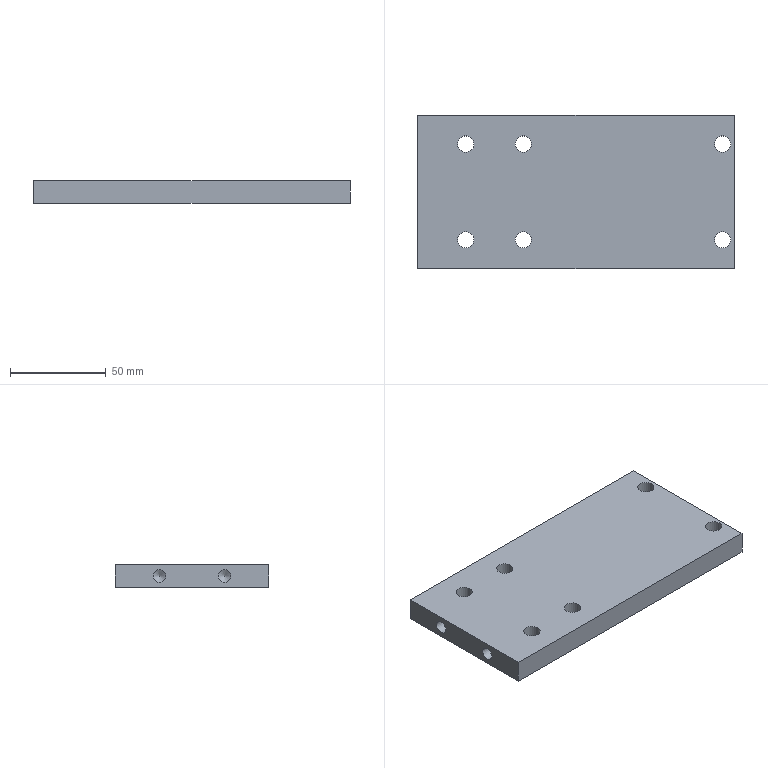Part | STEP file | SUPORTE | 1 solid | 16 faces | box 165 x 80 x 12 mm | volume 153227 mm3 | cylinder 8 | plane 6 | cone 2 | commonest cylinder face diameters 8.5 x6 6.647 x2
STEP:
#1=CARTESIAN_POINT('',(0.,0.,0.));
#2=DIRECTION('',(0.,0.,1.));
#3=DIRECTION('',(1.,0.,0.));
#4=AXIS2_PLACEMENT_3D('',#1,#2,#3);
#5=CARTESIAN_POINT('',(-206.95,452.,9.323));
#6=VERTEX_POINT('',#5);
#7=CARTESIAN_POINT('',(-206.95,452.,6.));
#8=DIRECTION('',(-1.,0.,0.));
#9=DIRECTION('',(0.,0.,1.));
#10=AXIS2_PLACEMENT_3D('',#7,#8,#9);
#11=CIRCLE('',#10,3.324);
#12=CARTESIAN_POINT('',(-205.952,452.,6.));
#13=DIRECTION('',(-1.,0.,0.));
#14=DIRECTION('',(0.,0.,1.));
#15=AXIS2_PLACEMENT_3D('',#12,#13,#14);
#16=CONICAL_SURFACE('',#15,1.662,1.03);
#17=CARTESIAN_POINT('',(0.,0.9985));
#18=DIRECTION('',(1.,0.));
#19=VECTOR('',#18,1.);
#20=LINE('',#17,#19);
#21=(GEOMETRIC_REPRESENTATION_CONTEXT(2)PARAMETRIC_REPRESENTATION_CONTEXT()REPRESENTATION_CONTEXT('',''));
#22=DEFINITIONAL_REPRESENTATION('',(#20),#21);
#23=PCURVE('',#16,#22);
#24=CARTESIAN_POINT('',(-214.45,452.,6.));
#25=DIRECTION('',(-1.,0.,0.));
#26=DIRECTION('',(0.,0.,1.));
#27=AXIS2_PLACEMENT_3D('',#24,#25,#26);
#28=CYLINDRICAL_SURFACE('',#27,3.324);
#29=CARTESIAN_POINT('',(0.,-7.5));
#30=DIRECTION('',(1.,0.));
#31=VECTOR('',#30,1.);
#32=LINE('',#29,#31);
#33=(GEOMETRIC_REPRESENTATION_CONTEXT(2)PARAMETRIC_REPRESENTATION_CONTEXT()REPRESENTATION_CONTEXT('',''));
#34=DEFINITIONAL_REPRESENTATION('',(#32),#33);
#35=PCURVE('',#28,#34);
#36=SURFACE_CURVE('',#11,(#23,#35),.PCURVE_S1.);
#37=EDGE_CURVE('',#6,#6,#36,.T.);
#38=ORIENTED_EDGE('',*,*,#37,.F.);
#39=CARTESIAN_POINT('',(-204.953,452.,6.));
#40=VERTEX_POINT('',#39);
#41=CARTESIAN_POINT('',(-204.953,452.,6.));
#42=CARTESIAN_POINT('',(-206.95,452.,9.323));
#43=B_SPLINE_CURVE_WITH_KNOTS('',1,(#41,#42),.UNSPECIFIED.,.F.,.F.,(2,2),(-1.939,1.939),.PIECEWISE_BEZIER_KNOTS.);
#44=CARTESIAN_POINT('',(0.,0.));
#45=DIRECTION('',(0.,1.));
#46=VECTOR('',#45,1.);
#47=LINE('',#44,#46);
#48=(GEOMETRIC_REPRESENTATION_CONTEXT(2)PARAMETRIC_REPRESENTATION_CONTEXT()REPRESENTATION_CONTEXT('',''));
#49=DEFINITIONAL_REPRESENTATION('',(#47),#48);
#50=PCURVE('',#16,#49);
#51=CARTESIAN_POINT('',(6.283,0.));
#52=DIRECTION('',(0.,1.));
#53=VECTOR('',#52,1.);
#54=LINE('',#51,#53);
#55=(GEOMETRIC_REPRESENTATION_CONTEXT(2)PARAMETRIC_REPRESENTATION_CONTEXT()REPRESENTATION_CONTEXT('',''));
#56=DEFINITIONAL_REPRESENTATION('',(#54),#55);
#57=PCURVE('',#16,#56);
#58=SEAM_CURVE('',#43,(#50,#57),.PCURVE_S1.);
#59=EDGE_CURVE('',#40,#6,#58,.T.);
#60=ORIENTED_EDGE('',*,*,#59,.F.);
#61=ORIENTED_EDGE('',*,*,#59,.T.);
#62=EDGE_LOOP('',(#38,#60,#61));
#63=FACE_BOUND('',#62,.F.);
#64=ADVANCED_FACE('',(#63),#16,.F.);
#65=CARTESIAN_POINT('',(-221.95,452.,9.323));
#66=VERTEX_POINT('',#65);
#67=CARTESIAN_POINT('',(-221.95,452.,6.));
#68=DIRECTION('',(1.,0.,0.));
#69=DIRECTION('',(0.,0.,1.));
#70=AXIS2_PLACEMENT_3D('',#67,#68,#69);
#71=CIRCLE('',#70,3.324);
#72=CARTESIAN_POINT('',(6.283,7.5));
#73=DIRECTION('',(-1.,0.));
#74=VECTOR('',#73,1.);
#75=LINE('',#72,#74);
#76=(GEOMETRIC_REPRESENTATION_CONTEXT(2)PARAMETRIC_REPRESENTATION_CONTEXT()REPRESENTATION_CONTEXT('',''));
#77=DEFINITIONAL_REPRESENTATION('',(#75),#76);
#78=PCURVE('',#28,#77);
#79=CARTESIAN_POINT('',(-221.95,435.,6.));
#80=DIRECTION('',(1.,0.,0.));
#81=DIRECTION('',(0.,0.,-1.));
#82=AXIS2_PLACEMENT_3D('',#79,#80,#81);
#83=PLANE('',#82);
#84=CARTESIAN_POINT('',(0.,17.));
#85=DIRECTION('',(-1.,0.));
#86=AXIS2_PLACEMENT_2D('',#84,#85);
#87=CIRCLE('',#86,3.324);
#88=(GEOMETRIC_REPRESENTATION_CONTEXT(2)PARAMETRIC_REPRESENTATION_CONTEXT()REPRESENTATION_CONTEXT('',''));
#89=DEFINITIONAL_REPRESENTATION('',(#87),#88);
#90=PCURVE('',#83,#89);
#91=SURFACE_CURVE('',#71,(#78,#90),.PCURVE_S1.);
#92=EDGE_CURVE('',#66,#66,#91,.T.);
#93=ORIENTED_EDGE('',*,*,#92,.T.);
#94=CARTESIAN_POINT('',(-206.95,452.,9.323));
#95=CARTESIAN_POINT('',(-221.95,452.,9.323));
#96=B_SPLINE_CURVE_WITH_KNOTS('',1,(#94,#95),.UNSPECIFIED.,.F.,.F.,(2,2),(-7.5,7.5),.PIECEWISE_BEZIER_KNOTS.);
#97=CARTESIAN_POINT('',(0.,0.));
#98=DIRECTION('',(0.,1.));
#99=VECTOR('',#98,1.);
#100=LINE('',#97,#99);
#101=(GEOMETRIC_REPRESENTATION_CONTEXT(2)PARAMETRIC_REPRESENTATION_CONTEXT()REPRESENTATION_CONTEXT('',''));
#102=DEFINITIONAL_REPRESENTATION('',(#100),#101);
#103=PCURVE('',#28,#102);
#104=CARTESIAN_POINT('',(6.283,0.));
#105=DIRECTION('',(0.,1.));
#106=VECTOR('',#105,1.);
#107=LINE('',#104,#106);
#108=(GEOMETRIC_REPRESENTATION_CONTEXT(2)PARAMETRIC_REPRESENTATION_CONTEXT()REPRESENTATION_CONTEXT('',''));
#109=DEFINITIONAL_REPRESENTATION('',(#107),#108);
#110=PCURVE('',#28,#109);
#111=SEAM_CURVE('',#96,(#103,#110),.PCURVE_S1.);
#112=EDGE_CURVE('',#6,#66,#111,.T.);
#113=ORIENTED_EDGE('',*,*,#112,.F.);
#114=ORIENTED_EDGE('',*,*,#37,.T.);
#115=ORIENTED_EDGE('',*,*,#112,.T.);
#116=EDGE_LOOP('',(#93,#113,#114,#115));
#117=FACE_BOUND('',#116,.F.);
#118=ADVANCED_FACE('',(#117),#28,.F.);
#119=CARTESIAN_POINT('',(-206.95,418.,9.323));
#120=VERTEX_POINT('',#119);
#121=CARTESIAN_POINT('',(-206.95,418.,6.));
#122=DIRECTION('',(-1.,0.,0.));
#123=DIRECTION('',(0.,0.,1.));
#124=AXIS2_PLACEMENT_3D('',#121,#122,#123);
#125=CIRCLE('',#124,3.324);
#126=CARTESIAN_POINT('',(-205.952,418.,6.));
#127=DIRECTION('',(-1.,0.,0.));
#128=DIRECTION('',(0.,0.,1.));
#129=AXIS2_PLACEMENT_3D('',#126,#127,#128);
#130=CONICAL_SURFACE('',#129,1.662,1.03);
#131=CARTESIAN_POINT('',(0.,0.9985));
#132=DIRECTION('',(1.,0.));
#133=VECTOR('',#132,1.);
#134=LINE('',#131,#133);
#135=(GEOMETRIC_REPRESENTATION_CONTEXT(2)PARAMETRIC_REPRESENTATION_CONTEXT()REPRESENTATION_CONTEXT('',''));
#136=DEFINITIONAL_REPRESENTATION('',(#134),#135);
#137=PCURVE('',#130,#136);
#138=CARTESIAN_POINT('',(-214.45,418.,6.));
#139=DIRECTION('',(-1.,0.,0.));
#140=DIRECTION('',(0.,0.,1.));
#141=AXIS2_PLACEMENT_3D('',#138,#139,#140);
#142=CYLINDRICAL_SURFACE('',#141,3.324);
#143=CARTESIAN_POINT('',(0.,-7.5));
#144=DIRECTION('',(1.,0.));
#145=VECTOR('',#144,1.);
#146=LINE('',#143,#145);
#147=(GEOMETRIC_REPRESENTATION_CONTEXT(2)PARAMETRIC_REPRESENTATION_CONTEXT()REPRESENTATION_CONTEXT('',''));
#148=DEFINITIONAL_REPRESENTATION('',(#146),#147);
#149=PCURVE('',#142,#148);
#150=SURFACE_CURVE('',#125,(#137,#149),.PCURVE_S1.);
#151=EDGE_CURVE('',#120,#120,#150,.T.);
#152=ORIENTED_EDGE('',*,*,#151,.F.);
#153=CARTESIAN_POINT('',(-204.953,418.,6.));
#154=VERTEX_POINT('',#153);
#155=CARTESIAN_POINT('',(-204.953,418.,6.));
#156=CARTESIAN_POINT('',(-206.95,418.,9.323));
#157=B_SPLINE_CURVE_WITH_KNOTS('',1,(#155,#156),.UNSPECIFIED.,.F.,.F.,(2,2),(-1.939,1.939),.PIECEWISE_BEZIER_KNOTS.);
#158=CARTESIAN_POINT('',(0.,0.));
#159=DIRECTION('',(0.,1.));
#160=VECTOR('',#159,1.);
#161=LINE('',#158,#160);
#162=(GEOMETRIC_REPRESENTATION_CONTEXT(2)PARAMETRIC_REPRESENTATION_CONTEXT()REPRESENTATION_CONTEXT('',''));
#163=DEFINITIONAL_REPRESENTATION('',(#161),#162);
#164=PCURVE('',#130,#163);
#165=CARTESIAN_POINT('',(6.283,0.));
#166=DIRECTION('',(0.,1.));
#167=VECTOR('',#166,1.);
#168=LINE('',#165,#167);
#169=(GEOMETRIC_REPRESENTATION_CONTEXT(2)PARAMETRIC_REPRESENTATION_CONTEXT()REPRESENTATION_CONTEXT('',''));
#170=DEFINITIONAL_REPRESENTATION('',(#168),#169);
#171=PCURVE('',#130,#170);
#172=SEAM_CURVE('',#157,(#164,#171),.PCURVE_S1.);
#173=EDGE_CURVE('',#154,#120,#172,.T.);
#174=ORIENTED_EDGE('',*,*,#173,.F.);
#175=ORIENTED_EDGE('',*,*,#173,.T.);
#176=EDGE_LOOP('',(#152,#174,#175));
#177=FACE_BOUND('',#176,.F.);
#178=ADVANCED_FACE('',(#177),#130,.F.);
#179=CARTESIAN_POINT('',(-221.95,418.,9.323));
#180=VERTEX_POINT('',#179);
#181=CARTESIAN_POINT('',(-221.95,418.,6.));
#182=DIRECTION('',(1.,0.,0.));
#183=DIRECTION('',(0.,0.,1.));
#184=AXIS2_PLACEMENT_3D('',#181,#182,#183);
#185=CIRCLE('',#184,3.324);
#186=CARTESIAN_POINT('',(6.283,7.5));
#187=DIRECTION('',(-1.,0.));
#188=VECTOR('',#187,1.);
#189=LINE('',#186,#188);
#190=(GEOMETRIC_REPRESENTATION_CONTEXT(2)PARAMETRIC_REPRESENTATION_CONTEXT()REPRESENTATION_CONTEXT('',''));
#191=DEFINITIONAL_REPRESENTATION('',(#189),#190);
#192=PCURVE('',#142,#191);
#193=CARTESIAN_POINT('',(0.,-17.));
#194=DIRECTION('',(-1.,0.));
#195=AXIS2_PLACEMENT_2D('',#193,#194);
#196=CIRCLE('',#195,3.324);
#197=(GEOMETRIC_REPRESENTATION_CONTEXT(2)PARAMETRIC_REPRESENTATION_CONTEXT()REPRESENTATION_CONTEXT('',''));
#198=DEFINITIONAL_REPRESENTATION('',(#196),#197);
#199=PCURVE('',#83,#198);
#200=SURFACE_CURVE('',#185,(#192,#199),.PCURVE_S1.);
#201=EDGE_CURVE('',#180,#180,#200,.T.);
#202=ORIENTED_EDGE('',*,*,#201,.T.);
#203=CARTESIAN_POINT('',(-206.95,418.,9.323));
#204=CARTESIAN_POINT('',(-221.95,418.,9.323));
#205=B_SPLINE_CURVE_WITH_KNOTS('',1,(#203,#204),.UNSPECIFIED.,.F.,.F.,(2,2),(-7.5,7.5),.PIECEWISE_BEZIER_KNOTS.);
#206=CARTESIAN_POINT('',(0.,0.));
#207=DIRECTION('',(0.,1.));
#208=VECTOR('',#207,1.);
#209=LINE('',#206,#208);
#210=(GEOMETRIC_REPRESENTATION_CONTEXT(2)PARAMETRIC_REPRESENTATION_CONTEXT()REPRESENTATION_CONTEXT('',''));
#211=DEFINITIONAL_REPRESENTATION('',(#209),#210);
#212=PCURVE('',#142,#211);
#213=CARTESIAN_POINT('',(6.283,0.));
#214=DIRECTION('',(0.,1.));
#215=VECTOR('',#214,1.);
#216=LINE('',#213,#215);
#217=(GEOMETRIC_REPRESENTATION_CONTEXT(2)PARAMETRIC_REPRESENTATION_CONTEXT()REPRESENTATION_CONTEXT('',''));
#218=DEFINITIONAL_REPRESENTATION('',(#216),#217);
#219=PCURVE('',#142,#218);
#220=SEAM_CURVE('',#205,(#212,#219),.PCURVE_S1.);
#221=EDGE_CURVE('',#120,#180,#220,.T.);
#222=ORIENTED_EDGE('',*,*,#221,.F.);
#223=ORIENTED_EDGE('',*,*,#151,.T.);
#224=ORIENTED_EDGE('',*,*,#221,.T.);
#225=EDGE_LOOP('',(#202,#222,#223,#224));
#226=FACE_BOUND('',#225,.F.);
#227=ADVANCED_FACE('',(#226),#142,.F.);
#228=CARTESIAN_POINT('',(-221.95,395.,12.));
#229=VERTEX_POINT('',#228);
#230=CARTESIAN_POINT('',(-221.95,395.,0.));
#231=VERTEX_POINT('',#230);
#232=CARTESIAN_POINT('',(-221.95,395.,12.));
#233=DIRECTION('',(0.,0.,-1.));
#234=VECTOR('',#233,1.);
#235=LINE('',#232,#234);
#236=CARTESIAN_POINT('',(-6.,-40.));
#237=DIRECTION('',(1.,0.));
#238=VECTOR('',#237,1.);
#239=LINE('',#236,#238);
#240=(GEOMETRIC_REPRESENTATION_CONTEXT(2)PARAMETRIC_REPRESENTATION_CONTEXT()REPRESENTATION_CONTEXT('',''));
#241=DEFINITIONAL_REPRESENTATION('',(#239),#240);
#242=PCURVE('',#83,#241);
#243=CARTESIAN_POINT('',(-56.95,395.,0.));
#244=DIRECTION('',(0.,-1.,0.));
#245=DIRECTION('',(0.,0.,-1.));
#246=AXIS2_PLACEMENT_3D('',#243,#244,#245);
#247=PLANE('',#246);
#248=CARTESIAN_POINT('',(-12.,-165.));
#249=DIRECTION('',(1.,0.));
#250=VECTOR('',#249,1.);
#251=LINE('',#248,#250);
#252=(GEOMETRIC_REPRESENTATION_CONTEXT(2)PARAMETRIC_REPRESENTATION_CONTEXT()REPRESENTATION_CONTEXT('',''));
#253=DEFINITIONAL_REPRESENTATION('',(#251),#252);
#254=PCURVE('',#247,#253);
#255=SURFACE_CURVE('',#235,(#242,#254),.PCURVE_S1.);
#256=EDGE_CURVE('',#229,#231,#255,.T.);
#257=ORIENTED_EDGE('',*,*,#256,.F.);
#258=CARTESIAN_POINT('',(-221.95,475.,12.));
#259=VERTEX_POINT('',#258);
#260=CARTESIAN_POINT('',(-221.95,475.,12.));
#261=DIRECTION('',(0.,-1.,0.));
#262=VECTOR('',#261,1.);
#263=LINE('',#260,#262);
#264=CARTESIAN_POINT('',(-6.,40.));
#265=DIRECTION('',(0.,-1.));
#266=VECTOR('',#265,1.);
#267=LINE('',#264,#266);
#268=(GEOMETRIC_REPRESENTATION_CONTEXT(2)PARAMETRIC_REPRESENTATION_CONTEXT()REPRESENTATION_CONTEXT('',''));
#269=DEFINITIONAL_REPRESENTATION('',(#267),#268);
#270=PCURVE('',#83,#269);
#271=CARTESIAN_POINT('',(-131.95,435.,12.));
#272=DIRECTION('',(0.,0.,1.));
#273=DIRECTION('',(1.,0.,0.));
#274=AXIS2_PLACEMENT_3D('',#271,#272,#273);
#275=PLANE('',#274);
#276=CARTESIAN_POINT('',(-90.,40.));
#277=DIRECTION('',(0.,-1.));
#278=VECTOR('',#277,1.);
#279=LINE('',#276,#278);
#280=(GEOMETRIC_REPRESENTATION_CONTEXT(2)PARAMETRIC_REPRESENTATION_CONTEXT()REPRESENTATION_CONTEXT('',''));
#281=DEFINITIONAL_REPRESENTATION('',(#279),#280);
#282=PCURVE('',#275,#281);
#283=SURFACE_CURVE('',#263,(#270,#282),.PCURVE_S1.);
#284=EDGE_CURVE('',#259,#229,#283,.T.);
#285=ORIENTED_EDGE('',*,*,#284,.F.);
#286=CARTESIAN_POINT('',(-221.95,475.,0.));
#287=VERTEX_POINT('',#286);
#288=CARTESIAN_POINT('',(-221.95,475.,0.));
#289=DIRECTION('',(0.,0.,1.));
#290=VECTOR('',#289,1.);
#291=LINE('',#288,#290);
#292=CARTESIAN_POINT('',(6.,40.));
#293=DIRECTION('',(-1.,0.));
#294=VECTOR('',#293,1.);
#295=LINE('',#292,#294);
#296=(GEOMETRIC_REPRESENTATION_CONTEXT(2)PARAMETRIC_REPRESENTATION_CONTEXT()REPRESENTATION_CONTEXT('',''));
#297=DEFINITIONAL_REPRESENTATION('',(#295),#296);
#298=PCURVE('',#83,#297);
#299=CARTESIAN_POINT('',(-206.95,475.,0.));
#300=DIRECTION('',(0.,1.,0.));
#301=DIRECTION('',(0.,0.,1.));
#302=AXIS2_PLACEMENT_3D('',#299,#300,#301);
#303=PLANE('',#302);
#304=CARTESIAN_POINT('',(0.,-15.));
#305=DIRECTION('',(1.,0.));
#306=VECTOR('',#305,1.);
#307=LINE('',#304,#306);
#308=(GEOMETRIC_REPRESENTATION_CONTEXT(2)PARAMETRIC_REPRESENTATION_CONTEXT()REPRESENTATION_CONTEXT('',''));
#309=DEFINITIONAL_REPRESENTATION('',(#307),#308);
#310=PCURVE('',#303,#309);
#311=SURFACE_CURVE('',#291,(#298,#310),.PCURVE_S1.);
#312=EDGE_CURVE('',#287,#259,#311,.T.);
#313=ORIENTED_EDGE('',*,*,#312,.F.);
#314=CARTESIAN_POINT('',(-221.95,395.,0.));
#315=DIRECTION('',(0.,1.,0.));
#316=VECTOR('',#315,1.);
#317=LINE('',#314,#316);
#318=CARTESIAN_POINT('',(6.,-40.));
#319=DIRECTION('',(0.,1.));
#320=VECTOR('',#319,1.);
#321=LINE('',#318,#320);
#322=(GEOMETRIC_REPRESENTATION_CONTEXT(2)PARAMETRIC_REPRESENTATION_CONTEXT()REPRESENTATION_CONTEXT('',''));
#323=DEFINITIONAL_REPRESENTATION('',(#321),#322);
#324=PCURVE('',#83,#323);
#325=CARTESIAN_POINT('',(-131.95,435.,0.));
#326=DIRECTION('',(0.,0.,1.));
#327=DIRECTION('',(1.,0.,0.));
#328=AXIS2_PLACEMENT_3D('',#325,#326,#327);
#329=PLANE('',#328);
#330=CARTESIAN_POINT('',(-90.,-40.));
#331=DIRECTION('',(0.,1.));
#332=VECTOR('',#331,1.);
#333=LINE('',#330,#332);
#334=(GEOMETRIC_REPRESENTATION_CONTEXT(2)PARAMETRIC_REPRESENTATION_CONTEXT()REPRESENTATION_CONTEXT('',''));
#335=DEFINITIONAL_REPRESENTATION('',(#333),#334);
#336=PCURVE('',#329,#335);
#337=SURFACE_CURVE('',#317,(#324,#336),.PCURVE_S1.);
#338=EDGE_CURVE('',#231,#287,#337,.T.);
#339=ORIENTED_EDGE('',*,*,#338,.F.);
#340=EDGE_LOOP('',(#257,#285,#313,#339));
#341=FACE_BOUND('',#340,.T.);
#342=ORIENTED_EDGE('',*,*,#92,.T.);
#343=EDGE_LOOP('',(#342));
#344=FACE_BOUND('',#343,.T.);
#345=ORIENTED_EDGE('',*,*,#201,.T.);
#346=EDGE_LOOP('',(#345));
#347=FACE_BOUND('',#346,.T.);
#348=ADVANCED_FACE('',(#341,#344,#347),#83,.F.);
#349=CARTESIAN_POINT('',(-171.2,460.,0.));
#350=VERTEX_POINT('',#349);
#351=CARTESIAN_POINT('',(-162.7,460.,0.));
#352=VERTEX_POINT('',#351);
#353=CARTESIAN_POINT('',(-166.95,460.,0.));
#354=DIRECTION('',(0.,0.,1.));
#355=DIRECTION('',(1.,0.,0.));
#356=AXIS2_PLACEMENT_3D('',#353,#354,#355);
#357=CIRCLE('',#356,4.25);
#358=CARTESIAN_POINT('',(-166.95,460.,-158.423));
#359=DIRECTION('',(0.,0.,1.));
#360=DIRECTION('',(1.,0.,0.));
#361=AXIS2_PLACEMENT_3D('',#358,#359,#360);
#362=CYLINDRICAL_SURFACE('',#361,4.25);
#363=CARTESIAN_POINT('',(0.,158.423));
#364=DIRECTION('',(1.,0.));
#365=VECTOR('',#364,1.);
#366=LINE('',#363,#365);
#367=(GEOMETRIC_REPRESENTATION_CONTEXT(2)PARAMETRIC_REPRESENTATION_CONTEXT()REPRESENTATION_CONTEXT('',''));
#368=DEFINITIONAL_REPRESENTATION('',(#366),#367);
#369=PCURVE('',#362,#368);
#370=CARTESIAN_POINT('',(-35.,25.));
#371=DIRECTION('',(1.,0.));
#372=AXIS2_PLACEMENT_2D('',#370,#371);
#373=CIRCLE('',#372,4.25);
#374=(GEOMETRIC_REPRESENTATION_CONTEXT(2)PARAMETRIC_REPRESENTATION_CONTEXT()REPRESENTATION_CONTEXT('',''));
#375=DEFINITIONAL_REPRESENTATION('',(#373),#374);
#376=PCURVE('',#329,#375);
#377=SURFACE_CURVE('',#357,(#369,#376),.PCURVE_S1.);
#378=EDGE_CURVE('',#350,#352,#377,.T.);
#379=ORIENTED_EDGE('',*,*,#378,.T.);
#380=CARTESIAN_POINT('',(-162.7,460.,12.));
#381=VERTEX_POINT('',#380);
#382=CARTESIAN_POINT('',(-162.7,460.,0.));
#383=CARTESIAN_POINT('',(-162.7,460.,12.));
#384=B_SPLINE_CURVE_WITH_KNOTS('',1,(#382,#383),.UNSPECIFIED.,.F.,.F.,(2,2),(158.423,170.423),.PIECEWISE_BEZIER_KNOTS.);
#385=CARTESIAN_POINT('',(6.283,0.));
#386=DIRECTION('',(0.,1.));
#387=VECTOR('',#386,1.);
#388=LINE('',#385,#387);
#389=(GEOMETRIC_REPRESENTATION_CONTEXT(2)PARAMETRIC_REPRESENTATION_CONTEXT()REPRESENTATION_CONTEXT('',''));
#390=DEFINITIONAL_REPRESENTATION('',(#388),#389);
#391=PCURVE('',#362,#390);
#392=CARTESIAN_POINT('',(0.,0.));
#393=DIRECTION('',(0.,1.));
#394=VECTOR('',#393,1.);
#395=LINE('',#392,#394);
#396=(GEOMETRIC_REPRESENTATION_CONTEXT(2)PARAMETRIC_REPRESENTATION_CONTEXT()REPRESENTATION_CONTEXT('',''));
#397=DEFINITIONAL_REPRESENTATION('',(#395),#396);
#398=PCURVE('',#362,#397);
#399=SEAM_CURVE('',#384,(#391,#398),.PCURVE_S1.);
#400=EDGE_CURVE('',#352,#381,#399,.T.);
#401=ORIENTED_EDGE('',*,*,#400,.T.);
#402=CARTESIAN_POINT('',(-166.95,460.,12.));
#403=DIRECTION('',(0.,0.,-1.));
#404=DIRECTION('',(1.,0.,0.));
#405=AXIS2_PLACEMENT_3D('',#402,#403,#404);
#406=CIRCLE('',#405,4.25);
#407=CARTESIAN_POINT('',(6.283,170.423));
#408=DIRECTION('',(-1.,0.));
#409=VECTOR('',#408,1.);
#410=LINE('',#407,#409);
#411=(GEOMETRIC_REPRESENTATION_CONTEXT(2)PARAMETRIC_REPRESENTATION_CONTEXT()REPRESENTATION_CONTEXT('',''));
#412=DEFINITIONAL_REPRESENTATION('',(#410),#411);
#413=PCURVE('',#362,#412);
#414=CARTESIAN_POINT('',(-30.75,25.));
#415=CARTESIAN_POINT('',(-30.75,17.639));
#416=CARTESIAN_POINT('',(-37.125,21.319));
#417=CARTESIAN_POINT('',(-43.5,25.));
#418=CARTESIAN_POINT('',(-37.125,28.681));
#419=CARTESIAN_POINT('',(-30.75,32.361));
#420=CARTESIAN_POINT('',(-30.75,25.));
#421=(BOUNDED_CURVE()B_SPLINE_CURVE(2,(#414,#415,#416,#417,#418,#419,#420),.UNSPECIFIED.,.T.,.F.)B_SPLINE_CURVE_WITH_KNOTS((1,2,2,2,2,1),(-2.094,0.,2.094,4.189,6.283,8.378),.UNSPECIFIED.)CURVE()GEOMETRIC_REPRESENTATION_ITEM()RATIONAL_B_SPLINE_CURVE((1.,0.5,1.,0.5,1.,0.5,1.))REPRESENTATION_ITEM(''));
#422=(GEOMETRIC_REPRESENTATION_CONTEXT(2)PARAMETRIC_REPRESENTATION_CONTEXT()REPRESENTATION_CONTEXT('',''));
#423=DEFINITIONAL_REPRESENTATION('',(#421),#422);
#424=PCURVE('',#275,#423);
#425=SURFACE_CURVE('',#406,(#413,#424),.PCURVE_S1.);
#426=EDGE_CURVE('',#381,#381,#425,.T.);
#427=ORIENTED_EDGE('',*,*,#426,.T.);
#428=ORIENTED_EDGE('',*,*,#400,.F.);
#429=CARTESIAN_POINT('',(-166.95,460.,0.));
#430=DIRECTION('',(0.,0.,1.));
#431=DIRECTION('',(1.,0.,0.));
#432=AXIS2_PLACEMENT_3D('',#429,#430,#431);
#433=CIRCLE('',#432,4.25);
#434=CARTESIAN_POINT('',(-6.283,158.423));
#435=DIRECTION('',(1.,0.));
#436=VECTOR('',#435,1.);
#437=LINE('',#434,#436);
#438=(GEOMETRIC_REPRESENTATION_CONTEXT(2)PARAMETRIC_REPRESENTATION_CONTEXT()REPRESENTATION_CONTEXT('',''));
#439=DEFINITIONAL_REPRESENTATION('',(#437),#438);
#440=PCURVE('',#362,#439);
#441=CARTESIAN_POINT('',(-35.,25.));
#442=DIRECTION('',(1.,0.));
#443=AXIS2_PLACEMENT_2D('',#441,#442);
#444=CIRCLE('',#443,4.25);
#445=(GEOMETRIC_REPRESENTATION_CONTEXT(2)PARAMETRIC_REPRESENTATION_CONTEXT()REPRESENTATION_CONTEXT('',''));
#446=DEFINITIONAL_REPRESENTATION('',(#444),#445);
#447=PCURVE('',#329,#446);
#448=SURFACE_CURVE('',#433,(#440,#447),.PCURVE_S1.);
#449=EDGE_CURVE('',#352,#350,#448,.T.);
#450=ORIENTED_EDGE('',*,*,#449,.T.);
#451=EDGE_LOOP('',(#379,#401,#427,#428,#450));
#452=FACE_BOUND('',#451,.F.);
#453=ADVANCED_FACE('',(#452),#362,.F.);
#454=CARTESIAN_POINT('',(-171.2,410.,0.));
#455=VERTEX_POINT('',#454);
#456=CARTESIAN_POINT('',(-162.7,410.,0.));
#457=VERTEX_POINT('',#456);
#458=CARTESIAN_POINT('',(-166.95,410.,0.));
#459=DIRECTION('',(0.,0.,1.));
#460=DIRECTION('',(1.,0.,0.));
#461=AXIS2_PLACEMENT_3D('',#458,#459,#460);
#462=CIRCLE('',#461,4.25);
#463=CARTESIAN_POINT('',(-166.95,410.,-158.423));
#464=DIRECTION('',(0.,0.,1.));
#465=DIRECTION('',(1.,0.,0.));
#466=AXIS2_PLACEMENT_3D('',#463,#464,#465);
#467=CYLINDRICAL_SURFACE('',#466,4.25);
#468=CARTESIAN_POINT('',(0.,158.423));
#469=DIRECTION('',(1.,0.));
#470=VECTOR('',#469,1.);
#471=LINE('',#468,#470);
#472=(GEOMETRIC_REPRESENTATION_CONTEXT(2)PARAMETRIC_REPRESENTATION_CONTEXT()REPRESENTATION_CONTEXT('',''));
#473=DEFINITIONAL_REPRESENTATION('',(#471),#472);
#474=PCURVE('',#467,#473);
#475=CARTESIAN_POINT('',(-35.,-25.));
#476=DIRECTION('',(1.,0.));
#477=AXIS2_PLACEMENT_2D('',#475,#476);
#478=CIRCLE('',#477,4.25);
#479=(GEOMETRIC_REPRESENTATION_CONTEXT(2)PARAMETRIC_REPRESENTATION_CONTEXT()REPRESENTATION_CONTEXT('',''));
#480=DEFINITIONAL_REPRESENTATION('',(#478),#479);
#481=PCURVE('',#329,#480);
#482=SURFACE_CURVE('',#462,(#474,#481),.PCURVE_S1.);
#483=EDGE_CURVE('',#455,#457,#482,.T.);
#484=ORIENTED_EDGE('',*,*,#483,.T.);
#485=CARTESIAN_POINT('',(-162.7,410.,12.));
#486=VERTEX_POINT('',#485);
#487=CARTESIAN_POINT('',(-162.7,410.,0.));
#488=CARTESIAN_POINT('',(-162.7,410.,12.));
#489=B_SPLINE_CURVE_WITH_KNOTS('',1,(#487,#488),.UNSPECIFIED.,.F.,.F.,(2,2),(158.423,170.423),.PIECEWISE_BEZIER_KNOTS.);
#490=CARTESIAN_POINT('',(6.283,0.));
#491=DIRECTION('',(0.,1.));
#492=VECTOR('',#491,1.);
#493=LINE('',#490,#492);
#494=(GEOMETRIC_REPRESENTATION_CONTEXT(2)PARAMETRIC_REPRESENTATION_CONTEXT()REPRESENTATION_CONTEXT('',''));
#495=DEFINITIONAL_REPRESENTATION('',(#493),#494);
#496=PCURVE('',#467,#495);
#497=CARTESIAN_POINT('',(0.,0.));
#498=DIRECTION('',(0.,1.));
#499=VECTOR('',#498,1.);
#500=LINE('',#497,#499);
#501=(GEOMETRIC_REPRESENTATION_CONTEXT(2)PARAMETRIC_REPRESENTATION_CONTEXT()REPRESENTATION_CONTEXT('',''));
#502=DEFINITIONAL_REPRESENTATION('',(#500),#501);
#503=PCURVE('',#467,#502);
#504=SEAM_CURVE('',#489,(#496,#503),.PCURVE_S1.);
#505=EDGE_CURVE('',#457,#486,#504,.T.);
#506=ORIENTED_EDGE('',*,*,#505,.T.);
#507=CARTESIAN_POINT('',(-166.95,410.,12.));
#508=DIRECTION('',(0.,0.,-1.));
#509=DIRECTION('',(1.,0.,0.));
#510=AXIS2_PLACEMENT_3D('',#507,#508,#509);
#511=CIRCLE('',#510,4.25);
#512=CARTESIAN_POINT('',(6.283,170.423));
#513=DIRECTION('',(-1.,0.));
#514=VECTOR('',#513,1.);
#515=LINE('',#512,#514);
#516=(GEOMETRIC_REPRESENTATION_CONTEXT(2)PARAMETRIC_REPRESENTATION_CONTEXT()REPRESENTATION_CONTEXT('',''));
#517=DEFINITIONAL_REPRESENTATION('',(#515),#516);
#518=PCURVE('',#467,#517);
#519=CARTESIAN_POINT('',(-30.75,-25.));
#520=CARTESIAN_POINT('',(-30.75,-32.361));
#521=CARTESIAN_POINT('',(-37.125,-28.681));
#522=CARTESIAN_POINT('',(-43.5,-25.));
#523=CARTESIAN_POINT('',(-37.125,-21.319));
#524=CARTESIAN_POINT('',(-30.75,-17.639));
#525=CARTESIAN_POINT('',(-30.75,-25.));
#526=(BOUNDED_CURVE()B_SPLINE_CURVE(2,(#519,#520,#521,#522,#523,#524,#525),.UNSPECIFIED.,.T.,.F.)B_SPLINE_CURVE_WITH_KNOTS((1,2,2,2,2,1),(-2.094,0.,2.094,4.189,6.283,8.378),.UNSPECIFIED.)CURVE()GEOMETRIC_REPRESENTATION_ITEM()RATIONAL_B_SPLINE_CURVE((1.,0.5,1.,0.5,1.,0.5,1.))REPRESENTATION_ITEM(''));
#527=(GEOMETRIC_REPRESENTATION_CONTEXT(2)PARAMETRIC_REPRESENTATION_CONTEXT()REPRESENTATION_CONTEXT('',''));
#528=DEFINITIONAL_REPRESENTATION('',(#526),#527);
#529=PCURVE('',#275,#528);
#530=SURFACE_CURVE('',#511,(#518,#529),.PCURVE_S1.);
#531=EDGE_CURVE('',#486,#486,#530,.T.);
#532=ORIENTED_EDGE('',*,*,#531,.T.);
#533=ORIENTED_EDGE('',*,*,#505,.F.);
#534=CARTESIAN_POINT('',(-166.95,410.,0.));
#535=DIRECTION('',(0.,0.,1.));
#536=DIRECTION('',(1.,0.,0.));
#537=AXIS2_PLACEMENT_3D('',#534,#535,#536);
#538=CIRCLE('',#537,4.25);
#539=CARTESIAN_POINT('',(-6.283,158.423));
#540=DIRECTION('',(1.,0.));
#541=VECTOR('',#540,1.);
#542=LINE('',#539,#541);
#543=(GEOMETRIC_REPRESENTATION_CONTEXT(2)PARAMETRIC_REPRESENTATION_CONTEXT()REPRESENTATION_CONTEXT('',''));
#544=DEFINITIONAL_REPRESENTATION('',(#542),#543);
#545=PCURVE('',#467,#544);
#546=CARTESIAN_POINT('',(-35.,-25.));
#547=DIRECTION('',(1.,0.));
#548=AXIS2_PLACEMENT_2D('',#546,#547);
#549=CIRCLE('',#548,4.25);
#550=(GEOMETRIC_REPRESENTATION_CONTEXT(2)PARAMETRIC_REPRESENTATION_CONTEXT()REPRESENTATION_CONTEXT('',''));
#551=DEFINITIONAL_REPRESENTATION('',(#549),#550);
#552=PCURVE('',#329,#551);
#553=SURFACE_CURVE('',#538,(#545,#552),.PCURVE_S1.);
#554=EDGE_CURVE('',#457,#455,#553,.T.);
#555=ORIENTED_EDGE('',*,*,#554,.T.);
#556=EDGE_LOOP('',(#484,#506,#532,#533,#555));
#557=FACE_BOUND('',#556,.F.);
#558=ADVANCED_FACE('',(#557),#467,.F.);
#559=CARTESIAN_POINT('',(-201.2,410.,0.));
#560=VERTEX_POINT('',#559);
#561=CARTESIAN_POINT('',(-192.7,410.,0.));
#562=VERTEX_POINT('',#561);
#563=CARTESIAN_POINT('',(-196.95,410.,0.));
#564=DIRECTION('',(0.,0.,1.));
#565=DIRECTION('',(1.,0.,0.));
#566=AXIS2_PLACEMENT_3D('',#563,#564,#565);
#567=CIRCLE('',#566,4.25);
#568=CARTESIAN_POINT('',(-196.95,410.,-158.423));
#569=DIRECTION('',(0.,0.,1.));
#570=DIRECTION('',(1.,0.,0.));
#571=AXIS2_PLACEMENT_3D('',#568,#569,#570);
#572=CYLINDRICAL_SURFACE('',#571,4.25);
#573=CARTESIAN_POINT('',(0.,158.423));
#574=DIRECTION('',(1.,0.));
#575=VECTOR('',#574,1.);
#576=LINE('',#573,#575);
#577=(GEOMETRIC_REPRESENTATION_CONTEXT(2)PARAMETRIC_REPRESENTATION_CONTEXT()REPRESENTATION_CONTEXT('',''));
#578=DEFINITIONAL_REPRESENTATION('',(#576),#577);
#579=PCURVE('',#572,#578);
#580=CARTESIAN_POINT('',(-65.,-25.));
#581=DIRECTION('',(1.,0.));
#582=AXIS2_PLACEMENT_2D('',#580,#581);
#583=CIRCLE('',#582,4.25);
#584=(GEOMETRIC_REPRESENTATION_CONTEXT(2)PARAMETRIC_REPRESENTATION_CONTEXT()REPRESENTATION_CONTEXT('',''));
#585=DEFINITIONAL_REPRESENTATION('',(#583),#584);
#586=PCURVE('',#329,#585);
#587=SURFACE_CURVE('',#567,(#579,#586),.PCURVE_S1.);
#588=EDGE_CURVE('',#560,#562,#587,.T.);
#589=ORIENTED_EDGE('',*,*,#588,.T.);
#590=CARTESIAN_POINT('',(-192.7,410.,12.));
#591=VERTEX_POINT('',#590);
#592=CARTESIAN_POINT('',(-192.7,410.,0.));
#593=CARTESIAN_POINT('',(-192.7,410.,12.));
#594=B_SPLINE_CURVE_WITH_KNOTS('',1,(#592,#593),.UNSPECIFIED.,.F.,.F.,(2,2),(158.423,170.423),.PIECEWISE_BEZIER_KNOTS.);
#595=CARTESIAN_POINT('',(6.283,0.));
#596=DIRECTION('',(0.,1.));
#597=VECTOR('',#596,1.);
#598=LINE('',#595,#597);
#599=(GEOMETRIC_REPRESENTATION_CONTEXT(2)PARAMETRIC_REPRESENTATION_CONTEXT()REPRESENTATION_CONTEXT('',''));
#600=DEFINITIONAL_REPRESENTATION('',(#598),#599);
#601=PCURVE('',#572,#600);
#602=CARTESIAN_POINT('',(0.,0.));
#603=DIRECTION('',(0.,1.));
#604=VECTOR('',#603,1.);
#605=LINE('',#602,#604);
#606=(GEOMETRIC_REPRESENTATION_CONTEXT(2)PARAMETRIC_REPRESENTATION_CONTEXT()REPRESENTATION_CONTEXT('',''));
#607=DEFINITIONAL_REPRESENTATION('',(#605),#606);
#608=PCURVE('',#572,#607);
#609=SEAM_CURVE('',#594,(#601,#608),.PCURVE_S1.);
#610=EDGE_CURVE('',#562,#591,#609,.T.);
#611=ORIENTED_EDGE('',*,*,#610,.T.);
#612=CARTESIAN_POINT('',(-196.95,410.,12.));
#613=DIRECTION('',(0.,0.,-1.));
#614=DIRECTION('',(1.,0.,0.));
#615=AXIS2_PLACEMENT_3D('',#612,#613,#614);
#616=CIRCLE('',#615,4.25);
#617=CARTESIAN_POINT('',(6.283,170.423));
#618=DIRECTION('',(-1.,0.));
#619=VECTOR('',#618,1.);
#620=LINE('',#617,#619);
#621=(GEOMETRIC_REPRESENTATION_CONTEXT(2)PARAMETRIC_REPRESENTATION_CONTEXT()REPRESENTATION_CONTEXT('',''));
#622=DEFINITIONAL_REPRESENTATION('',(#620),#621);
#623=PCURVE('',#572,#622);
#624=CARTESIAN_POINT('',(-60.75,-25.));
#625=CARTESIAN_POINT('',(-60.75,-32.361));
#626=CARTESIAN_POINT('',(-67.125,-28.681));
#627=CARTESIAN_POINT('',(-73.5,-25.));
#628=CARTESIAN_POINT('',(-67.125,-21.319));
#629=CARTESIAN_POINT('',(-60.75,-17.639));
#630=CARTESIAN_POINT('',(-60.75,-25.));
#631=(BOUNDED_CURVE()B_SPLINE_CURVE(2,(#624,#625,#626,#627,#628,#629,#630),.UNSPECIFIED.,.T.,.F.)B_SPLINE_CURVE_WITH_KNOTS((1,2,2,2,2,1),(-2.094,0.,2.094,4.189,6.283,8.378),.UNSPECIFIED.)CURVE()GEOMETRIC_REPRESENTATION_ITEM()RATIONAL_B_SPLINE_CURVE((1.,0.5,1.,0.5,1.,0.5,1.))REPRESENTATION_ITEM(''));
#632=(GEOMETRIC_REPRESENTATION_CONTEXT(2)PARAMETRIC_REPRESENTATION_CONTEXT()REPRESENTATION_CONTEXT('',''));
#633=DEFINITIONAL_REPRESENTATION('',(#631),#632);
#634=PCURVE('',#275,#633);
#635=SURFACE_CURVE('',#616,(#623,#634),.PCURVE_S1.);
#636=EDGE_CURVE('',#591,#591,#635,.T.);
#637=ORIENTED_EDGE('',*,*,#636,.T.);
#638=ORIENTED_EDGE('',*,*,#610,.F.);
#639=CARTESIAN_POINT('',(-196.95,410.,0.));
#640=DIRECTION('',(0.,0.,1.));
#641=DIRECTION('',(1.,0.,0.));
#642=AXIS2_PLACEMENT_3D('',#639,#640,#641);
#643=CIRCLE('',#642,4.25);
#644=CARTESIAN_POINT('',(-6.283,158.423));
#645=DIRECTION('',(1.,0.));
#646=VECTOR('',#645,1.);
#647=LINE('',#644,#646);
#648=(GEOMETRIC_REPRESENTATION_CONTEXT(2)PARAMETRIC_REPRESENTATION_CONTEXT()REPRESENTATION_CONTEXT('',''));
#649=DEFINITIONAL_REPRESENTATION('',(#647),#648);
#650=PCURVE('',#572,#649);
#651=CARTESIAN_POINT('',(-65.,-25.));
#652=DIRECTION('',(1.,0.));
#653=AXIS2_PLACEMENT_2D('',#651,#652);
#654=CIRCLE('',#653,4.25);
#655=(GEOMETRIC_REPRESENTATION_CONTEXT(2)PARAMETRIC_REPRESENTATION_CONTEXT()REPRESENTATION_CONTEXT('',''));
#656=DEFINITIONAL_REPRESENTATION('',(#654),#655);
#657=PCURVE('',#329,#656);
#658=SURFACE_CURVE('',#643,(#650,#657),.PCURVE_S1.);
#659=EDGE_CURVE('',#562,#560,#658,.T.);
#660=ORIENTED_EDGE('',*,*,#659,.T.);
#661=EDGE_LOOP('',(#589,#611,#637,#638,#660));
#662=FACE_BOUND('',#661,.F.);
#663=ADVANCED_FACE('',(#662),#572,.F.);
#664=CARTESIAN_POINT('',(-201.2,460.,0.));
#665=VERTEX_POINT('',#664);
#666=CARTESIAN_POINT('',(-192.7,460.,0.));
#667=VERTEX_POINT('',#666);
#668=CARTESIAN_POINT('',(-196.95,460.,0.));
#669=DIRECTION('',(0.,0.,1.));
#670=DIRECTION('',(1.,0.,0.));
#671=AXIS2_PLACEMENT_3D('',#668,#669,#670);
#672=CIRCLE('',#671,4.25);
#673=CARTESIAN_POINT('',(-196.95,460.,-158.423));
#674=DIRECTION('',(0.,0.,1.));
#675=DIRECTION('',(1.,0.,0.));
#676=AXIS2_PLACEMENT_3D('',#673,#674,#675);
#677=CYLINDRICAL_SURFACE('',#676,4.25);
#678=CARTESIAN_POINT('',(0.,158.423));
#679=DIRECTION('',(1.,0.));
#680=VECTOR('',#679,1.);
#681=LINE('',#678,#680);
#682=(GEOMETRIC_REPRESENTATION_CONTEXT(2)PARAMETRIC_REPRESENTATION_CONTEXT()REPRESENTATION_CONTEXT('',''));
#683=DEFINITIONAL_REPRESENTATION('',(#681),#682);
#684=PCURVE('',#677,#683);
#685=CARTESIAN_POINT('',(-65.,25.));
#686=DIRECTION('',(1.,0.));
#687=AXIS2_PLACEMENT_2D('',#685,#686);
#688=CIRCLE('',#687,4.25);
#689=(GEOMETRIC_REPRESENTATION_CONTEXT(2)PARAMETRIC_REPRESENTATION_CONTEXT()REPRESENTATION_CONTEXT('',''));
#690=DEFINITIONAL_REPRESENTATION('',(#688),#689);
#691=PCURVE('',#329,#690);
#692=SURFACE_CURVE('',#672,(#684,#691),.PCURVE_S1.);
#693=EDGE_CURVE('',#665,#667,#692,.T.);
#694=ORIENTED_EDGE('',*,*,#693,.T.);
#695=CARTESIAN_POINT('',(-192.7,460.,12.));
#696=VERTEX_POINT('',#695);
#697=CARTESIAN_POINT('',(-192.7,460.,0.));
#698=CARTESIAN_POINT('',(-192.7,460.,12.));
#699=B_SPLINE_CURVE_WITH_KNOTS('',1,(#697,#698),.UNSPECIFIED.,.F.,.F.,(2,2),(158.423,170.423),.PIECEWISE_BEZIER_KNOTS.);
#700=CARTESIAN_POINT('',(6.283,0.));
#701=DIRECTION('',(0.,1.));
#702=VECTOR('',#701,1.);
#703=LINE('',#700,#702);
#704=(GEOMETRIC_REPRESENTATION_CONTEXT(2)PARAMETRIC_REPRESENTATION_CONTEXT()REPRESENTATION_CONTEXT('',''));
#705=DEFINITIONAL_REPRESENTATION('',(#703),#704);
#706=PCURVE('',#677,#705);
#707=CARTESIAN_POINT('',(0.,0.));
#708=DIRECTION('',(0.,1.));
#709=VECTOR('',#708,1.);
#710=LINE('',#707,#709);
#711=(GEOMETRIC_REPRESENTATION_CONTEXT(2)PARAMETRIC_REPRESENTATION_CONTEXT()REPRESENTATION_CONTEXT('',''));
#712=DEFINITIONAL_REPRESENTATION('',(#710),#711);
#713=PCURVE('',#677,#712);
#714=SEAM_CURVE('',#699,(#706,#713),.PCURVE_S1.);
#715=EDGE_CURVE('',#667,#696,#714,.T.);
#716=ORIENTED_EDGE('',*,*,#715,.T.);
#717=CARTESIAN_POINT('',(-196.95,460.,12.));
#718=DIRECTION('',(0.,0.,-1.));
#719=DIRECTION('',(1.,0.,0.));
#720=AXIS2_PLACEMENT_3D('',#717,#718,#719);
#721=CIRCLE('',#720,4.25);
#722=CARTESIAN_POINT('',(6.283,170.423));
#723=DIRECTION('',(-1.,0.));
#724=VECTOR('',#723,1.);
#725=LINE('',#722,#724);
#726=(GEOMETRIC_REPRESENTATION_CONTEXT(2)PARAMETRIC_REPRESENTATION_CONTEXT()REPRESENTATION_CONTEXT('',''));
#727=DEFINITIONAL_REPRESENTATION('',(#725),#726);
#728=PCURVE('',#677,#727);
#729=CARTESIAN_POINT('',(-60.75,25.));
#730=CARTESIAN_POINT('',(-60.75,17.639));
#731=CARTESIAN_POINT('',(-67.125,21.319));
#732=CARTESIAN_POINT('',(-73.5,25.));
#733=CARTESIAN_POINT('',(-67.125,28.681));
#734=CARTESIAN_POINT('',(-60.75,32.361));
#735=CARTESIAN_POINT('',(-60.75,25.));
#736=(BOUNDED_CURVE()B_SPLINE_CURVE(2,(#729,#730,#731,#732,#733,#734,#735),.UNSPECIFIED.,.T.,.F.)B_SPLINE_CURVE_WITH_KNOTS((1,2,2,2,2,1),(-2.094,0.,2.094,4.189,6.283,8.378),.UNSPECIFIED.)CURVE()GEOMETRIC_REPRESENTATION_ITEM()RATIONAL_B_SPLINE_CURVE((1.,0.5,1.,0.5,1.,0.5,1.))REPRESENTATION_ITEM(''));
#737=(GEOMETRIC_REPRESENTATION_CONTEXT(2)PARAMETRIC_REPRESENTATION_CONTEXT()REPRESENTATION_CONTEXT('',''));
#738=DEFINITIONAL_REPRESENTATION('',(#736),#737);
#739=PCURVE('',#275,#738);
#740=SURFACE_CURVE('',#721,(#728,#739),.PCURVE_S1.);
#741=EDGE_CURVE('',#696,#696,#740,.T.);
#742=ORIENTED_EDGE('',*,*,#741,.T.);
#743=ORIENTED_EDGE('',*,*,#715,.F.);
#744=CARTESIAN_POINT('',(-196.95,460.,0.));
#745=DIRECTION('',(0.,0.,1.));
#746=DIRECTION('',(1.,0.,0.));
#747=AXIS2_PLACEMENT_3D('',#744,#745,#746);
#748=CIRCLE('',#747,4.25);
#749=CARTESIAN_POINT('',(-6.283,158.423));
#750=DIRECTION('',(1.,0.));
#751=VECTOR('',#750,1.);
#752=LINE('',#749,#751);
#753=(GEOMETRIC_REPRESENTATION_CONTEXT(2)PARAMETRIC_REPRESENTATION_CONTEXT()REPRESENTATION_CONTEXT('',''));
#754=DEFINITIONAL_REPRESENTATION('',(#752),#753);
#755=PCURVE('',#677,#754);
#756=CARTESIAN_POINT('',(-65.,25.));
#757=DIRECTION('',(1.,0.));
#758=AXIS2_PLACEMENT_2D('',#756,#757);
#759=CIRCLE('',#758,4.25);
#760=(GEOMETRIC_REPRESENTATION_CONTEXT(2)PARAMETRIC_REPRESENTATION_CONTEXT()REPRESENTATION_CONTEXT('',''));
#761=DEFINITIONAL_REPRESENTATION('',(#759),#760);
#762=PCURVE('',#329,#761);
#763=SURFACE_CURVE('',#748,(#755,#762),.PCURVE_S1.);
#764=EDGE_CURVE('',#667,#665,#763,.T.);
#765=ORIENTED_EDGE('',*,*,#764,.T.);
#766=EDGE_LOOP('',(#694,#716,#742,#743,#765));
#767=FACE_BOUND('',#766,.F.);
#768=ADVANCED_FACE('',(#767),#677,.F.);
#769=CARTESIAN_POINT('',(-67.2,460.,0.));
#770=VERTEX_POINT('',#769);
#771=CARTESIAN_POINT('',(-58.7,460.,0.));
#772=VERTEX_POINT('',#771);
#773=CARTESIAN_POINT('',(-62.95,460.,0.));
#774=DIRECTION('',(0.,0.,1.));
#775=DIRECTION('',(1.,0.,0.));
#776=AXIS2_PLACEMENT_3D('',#773,#774,#775);
#777=CIRCLE('',#776,4.25);
#778=CARTESIAN_POINT('',(-62.95,460.,-158.423));
#779=DIRECTION('',(0.,0.,1.));
#780=DIRECTION('',(1.,0.,0.));
#781=AXIS2_PLACEMENT_3D('',#778,#779,#780);
#782=CYLINDRICAL_SURFACE('',#781,4.25);
#783=CARTESIAN_POINT('',(0.,158.423));
#784=DIRECTION('',(1.,0.));
#785=VECTOR('',#784,1.);
#786=LINE('',#783,#785);
#787=(GEOMETRIC_REPRESENTATION_CONTEXT(2)PARAMETRIC_REPRESENTATION_CONTEXT()REPRESENTATION_CONTEXT('',''));
#788=DEFINITIONAL_REPRESENTATION('',(#786),#787);
#789=PCURVE('',#782,#788);
#790=CARTESIAN_POINT('',(69.,25.));
#791=DIRECTION('',(1.,0.));
#792=AXIS2_PLACEMENT_2D('',#790,#791);
#793=CIRCLE('',#792,4.25);
#794=(GEOMETRIC_REPRESENTATION_CONTEXT(2)PARAMETRIC_REPRESENTATION_CONTEXT()REPRESENTATION_CONTEXT('',''));
#795=DEFINITIONAL_REPRESENTATION('',(#793),#794);
#796=PCURVE('',#329,#795);
#797=SURFACE_CURVE('',#777,(#789,#796),.PCURVE_S1.);
#798=EDGE_CURVE('',#770,#772,#797,.T.);
#799=ORIENTED_EDGE('',*,*,#798,.T.);
#800=CARTESIAN_POINT('',(-58.7,460.,12.));
#801=VERTEX_POINT('',#800);
#802=CARTESIAN_POINT('',(-58.7,460.,0.));
#803=CARTESIAN_POINT('',(-58.7,460.,12.));
#804=B_SPLINE_CURVE_WITH_KNOTS('',1,(#802,#803),.UNSPECIFIED.,.F.,.F.,(2,2),(158.423,170.423),.PIECEWISE_BEZIER_KNOTS.);
#805=CARTESIAN_POINT('',(6.283,0.));
#806=DIRECTION('',(0.,1.));
#807=VECTOR('',#806,1.);
#808=LINE('',#805,#807);
#809=(GEOMETRIC_REPRESENTATION_CONTEXT(2)PARAMETRIC_REPRESENTATION_CONTEXT()REPRESENTATION_CONTEXT('',''));
#810=DEFINITIONAL_REPRESENTATION('',(#808),#809);
#811=PCURVE('',#782,#810);
#812=CARTESIAN_POINT('',(0.,0.));
#813=DIRECTION('',(0.,1.));
#814=VECTOR('',#813,1.);
#815=LINE('',#812,#814);
#816=(GEOMETRIC_REPRESENTATION_CONTEXT(2)PARAMETRIC_REPRESENTATION_CONTEXT()REPRESENTATION_CONTEXT('',''));
#817=DEFINITIONAL_REPRESENTATION('',(#815),#816);
#818=PCURVE('',#782,#817);
#819=SEAM_CURVE('',#804,(#811,#818),.PCURVE_S1.);
#820=EDGE_CURVE('',#772,#801,#819,.T.);
#821=ORIENTED_EDGE('',*,*,#820,.T.);
#822=CARTESIAN_POINT('',(-62.95,460.,12.));
#823=DIRECTION('',(0.,0.,-1.));
#824=DIRECTION('',(1.,0.,0.));
#825=AXIS2_PLACEMENT_3D('',#822,#823,#824);
#826=CIRCLE('',#825,4.25);
#827=CARTESIAN_POINT('',(6.283,170.423));
#828=DIRECTION('',(-1.,0.));
#829=VECTOR('',#828,1.);
#830=LINE('',#827,#829);
#831=(GEOMETRIC_REPRESENTATION_CONTEXT(2)PARAMETRIC_REPRESENTATION_CONTEXT()REPRESENTATION_CONTEXT('',''));
#832=DEFINITIONAL_REPRESENTATION('',(#830),#831);
#833=PCURVE('',#782,#832);
#834=CARTESIAN_POINT('',(73.25,25.));
#835=CARTESIAN_POINT('',(73.25,17.639));
#836=CARTESIAN_POINT('',(66.875,21.319));
#837=CARTESIAN_POINT('',(60.5,25.));
#838=CARTESIAN_POINT('',(66.875,28.681));
#839=CARTESIAN_POINT('',(73.25,32.361));
#840=CARTESIAN_POINT('',(73.25,25.));
#841=(BOUNDED_CURVE()B_SPLINE_CURVE(2,(#834,#835,#836,#837,#838,#839,#840),.UNSPECIFIED.,.T.,.F.)B_SPLINE_CURVE_WITH_KNOTS((1,2,2,2,2,1),(-2.094,0.,2.094,4.189,6.283,8.378),.UNSPECIFIED.)CURVE()GEOMETRIC_REPRESENTATION_ITEM()RATIONAL_B_SPLINE_CURVE((1.,0.5,1.,0.5,1.,0.5,1.))REPRESENTATION_ITEM(''));
#842=(GEOMETRIC_REPRESENTATION_CONTEXT(2)PARAMETRIC_REPRESENTATION_CONTEXT()REPRESENTATION_CONTEXT('',''));
#843=DEFINITIONAL_REPRESENTATION('',(#841),#842);
#844=PCURVE('',#275,#843);
#845=SURFACE_CURVE('',#826,(#833,#844),.PCURVE_S1.);
#846=EDGE_CURVE('',#801,#801,#845,.T.);
#847=ORIENTED_EDGE('',*,*,#846,.T.);
#848=ORIENTED_EDGE('',*,*,#820,.F.);
#849=CARTESIAN_POINT('',(-62.95,460.,0.));
#850=DIRECTION('',(0.,0.,1.));
#851=DIRECTION('',(1.,0.,0.));
#852=AXIS2_PLACEMENT_3D('',#849,#850,#851);
#853=CIRCLE('',#852,4.25);
#854=CARTESIAN_POINT('',(-6.283,158.423));
#855=DIRECTION('',(1.,0.));
#856=VECTOR('',#855,1.);
#857=LINE('',#854,#856);
#858=(GEOMETRIC_REPRESENTATION_CONTEXT(2)PARAMETRIC_REPRESENTATION_CONTEXT()REPRESENTATION_CONTEXT('',''));
#859=DEFINITIONAL_REPRESENTATION('',(#857),#858);
#860=PCURVE('',#782,#859);
#861=CARTESIAN_POINT('',(69.,25.));
#862=DIRECTION('',(1.,0.));
#863=AXIS2_PLACEMENT_2D('',#861,#862);
#864=CIRCLE('',#863,4.25);
#865=(GEOMETRIC_REPRESENTATION_CONTEXT(2)PARAMETRIC_REPRESENTATION_CONTEXT()REPRESENTATION_CONTEXT('',''));
#866=DEFINITIONAL_REPRESENTATION('',(#864),#865);
#867=PCURVE('',#329,#866);
#868=SURFACE_CURVE('',#853,(#860,#867),.PCURVE_S1.);
#869=EDGE_CURVE('',#772,#770,#868,.T.);
#870=ORIENTED_EDGE('',*,*,#869,.T.);
#871=EDGE_LOOP('',(#799,#821,#847,#848,#870));
#872=FACE_BOUND('',#871,.F.);
#873=ADVANCED_FACE('',(#872),#782,.F.);
#874=CARTESIAN_POINT('',(-67.2,410.,0.));
#875=VERTEX_POINT('',#874);
#876=CARTESIAN_POINT('',(-58.7,410.,0.));
#877=VERTEX_POINT('',#876);
#878=CARTESIAN_POINT('',(-62.95,410.,0.));
#879=DIRECTION('',(0.,0.,1.));
#880=DIRECTION('',(1.,0.,0.));
#881=AXIS2_PLACEMENT_3D('',#878,#879,#880);
#882=CIRCLE('',#881,4.25);
#883=CARTESIAN_POINT('',(-62.95,410.,-158.423));
#884=DIRECTION('',(0.,0.,1.));
#885=DIRECTION('',(1.,0.,0.));
#886=AXIS2_PLACEMENT_3D('',#883,#884,#885);
#887=CYLINDRICAL_SURFACE('',#886,4.25);
#888=CARTESIAN_POINT('',(0.,158.423));
#889=DIRECTION('',(1.,0.));
#890=VECTOR('',#889,1.);
#891=LINE('',#888,#890);
#892=(GEOMETRIC_REPRESENTATION_CONTEXT(2)PARAMETRIC_REPRESENTATION_CONTEXT()REPRESENTATION_CONTEXT('',''));
#893=DEFINITIONAL_REPRESENTATION('',(#891),#892);
#894=PCURVE('',#887,#893);
#895=CARTESIAN_POINT('',(69.,-25.));
#896=DIRECTION('',(1.,0.));
#897=AXIS2_PLACEMENT_2D('',#895,#896);
#898=CIRCLE('',#897,4.25);
#899=(GEOMETRIC_REPRESENTATION_CONTEXT(2)PARAMETRIC_REPRESENTATION_CONTEXT()REPRESENTATION_CONTEXT('',''));
#900=DEFINITIONAL_REPRESENTATION('',(#898),#899);
#901=PCURVE('',#329,#900);
#902=SURFACE_CURVE('',#882,(#894,#901),.PCURVE_S1.);
#903=EDGE_CURVE('',#875,#877,#902,.T.);
#904=ORIENTED_EDGE('',*,*,#903,.T.);
#905=CARTESIAN_POINT('',(-58.7,410.,12.));
#906=VERTEX_POINT('',#905);
#907=CARTESIAN_POINT('',(-58.7,410.,0.));
#908=CARTESIAN_POINT('',(-58.7,410.,12.));
#909=B_SPLINE_CURVE_WITH_KNOTS('',1,(#907,#908),.UNSPECIFIED.,.F.,.F.,(2,2),(158.423,170.423),.PIECEWISE_BEZIER_KNOTS.);
#910=CARTESIAN_POINT('',(6.283,0.));
#911=DIRECTION('',(0.,1.));
#912=VECTOR('',#911,1.);
#913=LINE('',#910,#912);
#914=(GEOMETRIC_REPRESENTATION_CONTEXT(2)PARAMETRIC_REPRESENTATION_CONTEXT()REPRESENTATION_CONTEXT('',''));
#915=DEFINITIONAL_REPRESENTATION('',(#913),#914);
#916=PCURVE('',#887,#915);
#917=CARTESIAN_POINT('',(0.,0.));
#918=DIRECTION('',(0.,1.));
#919=VECTOR('',#918,1.);
#920=LINE('',#917,#919);
#921=(GEOMETRIC_REPRESENTATION_CONTEXT(2)PARAMETRIC_REPRESENTATION_CONTEXT()REPRESENTATION_CONTEXT('',''));
#922=DEFINITIONAL_REPRESENTATION('',(#920),#921);
#923=PCURVE('',#887,#922);
#924=SEAM_CURVE('',#909,(#916,#923),.PCURVE_S1.);
#925=EDGE_CURVE('',#877,#906,#924,.T.);
#926=ORIENTED_EDGE('',*,*,#925,.T.);
#927=CARTESIAN_POINT('',(-62.95,410.,12.));
#928=DIRECTION('',(0.,0.,-1.));
#929=DIRECTION('',(1.,0.,0.));
#930=AXIS2_PLACEMENT_3D('',#927,#928,#929);
#931=CIRCLE('',#930,4.25);
#932=CARTESIAN_POINT('',(6.283,170.423));
#933=DIRECTION('',(-1.,0.));
#934=VECTOR('',#933,1.);
#935=LINE('',#932,#934);
#936=(GEOMETRIC_REPRESENTATION_CONTEXT(2)PARAMETRIC_REPRESENTATION_CONTEXT()REPRESENTATION_CONTEXT('',''));
#937=DEFINITIONAL_REPRESENTATION('',(#935),#936);
#938=PCURVE('',#887,#937);
#939=CARTESIAN_POINT('',(73.25,-25.));
#940=CARTESIAN_POINT('',(73.25,-32.361));
#941=CARTESIAN_POINT('',(66.875,-28.681));
#942=CARTESIAN_POINT('',(60.5,-25.));
#943=CARTESIAN_POINT('',(66.875,-21.319));
#944=CARTESIAN_POINT('',(73.25,-17.639));
#945=CARTESIAN_POINT('',(73.25,-25.));
#946=(BOUNDED_CURVE()B_SPLINE_CURVE(2,(#939,#940,#941,#942,#943,#944,#945),.UNSPECIFIED.,.T.,.F.)B_SPLINE_CURVE_WITH_KNOTS((1,2,2,2,2,1),(-2.094,0.,2.094,4.189,6.283,8.378),.UNSPECIFIED.)CURVE()GEOMETRIC_REPRESENTATION_ITEM()RATIONAL_B_SPLINE_CURVE((1.,0.5,1.,0.5,1.,0.5,1.))REPRESENTATION_ITEM(''));
#947=(GEOMETRIC_REPRESENTATION_CONTEXT(2)PARAMETRIC_REPRESENTATION_CONTEXT()REPRESENTATION_CONTEXT('',''));
#948=DEFINITIONAL_REPRESENTATION('',(#946),#947);
#949=PCURVE('',#275,#948);
#950=SURFACE_CURVE('',#931,(#938,#949),.PCURVE_S1.);
#951=EDGE_CURVE('',#906,#906,#950,.T.);
#952=ORIENTED_EDGE('',*,*,#951,.T.);
#953=ORIENTED_EDGE('',*,*,#925,.F.);
#954=CARTESIAN_POINT('',(-62.95,410.,0.));
#955=DIRECTION('',(0.,0.,1.));
#956=DIRECTION('',(1.,0.,0.));
#957=AXIS2_PLACEMENT_3D('',#954,#955,#956);
#958=CIRCLE('',#957,4.25);
#959=CARTESIAN_POINT('',(-6.283,158.423));
#960=DIRECTION('',(1.,0.));
#961=VECTOR('',#960,1.);
#962=LINE('',#959,#961);
#963=(GEOMETRIC_REPRESENTATION_CONTEXT(2)PARAMETRIC_REPRESENTATION_CONTEXT()REPRESENTATION_CONTEXT('',''));
#964=DEFINITIONAL_REPRESENTATION('',(#962),#963);
#965=PCURVE('',#887,#964);
#966=CARTESIAN_POINT('',(69.,-25.));
#967=DIRECTION('',(1.,0.));
#968=AXIS2_PLACEMENT_2D('',#966,#967);
#969=CIRCLE('',#968,4.25);
#970=(GEOMETRIC_REPRESENTATION_CONTEXT(2)PARAMETRIC_REPRESENTATION_CONTEXT()REPRESENTATION_CONTEXT('',''));
#971=DEFINITIONAL_REPRESENTATION('',(#969),#970);
#972=PCURVE('',#329,#971);
#973=SURFACE_CURVE('',#958,(#965,#972),.PCURVE_S1.);
#974=EDGE_CURVE('',#877,#875,#973,.T.);
#975=ORIENTED_EDGE('',*,*,#974,.T.);
#976=EDGE_LOOP('',(#904,#926,#952,#953,#975));
#977=FACE_BOUND('',#976,.F.);
#978=ADVANCED_FACE('',(#977),#887,.F.);
#979=CARTESIAN_POINT('',(-56.95,475.,12.));
#980=VERTEX_POINT('',#979);
#981=CARTESIAN_POINT('',(-221.95,475.,12.));
#982=DIRECTION('',(1.,0.,0.));
#983=VECTOR('',#982,1.);
#984=LINE('',#981,#983);
#985=CARTESIAN_POINT('',(12.,-15.));
#986=DIRECTION('',(0.,1.));
#987=VECTOR('',#986,1.);
#988=LINE('',#985,#987);
#989=(GEOMETRIC_REPRESENTATION_CONTEXT(2)PARAMETRIC_REPRESENTATION_CONTEXT()REPRESENTATION_CONTEXT('',''));
#990=DEFINITIONAL_REPRESENTATION('',(#988),#989);
#991=PCURVE('',#303,#990);
#992=CARTESIAN_POINT('',(-90.,40.));
#993=DIRECTION('',(1.,0.));
#994=VECTOR('',#993,1.);
#995=LINE('',#992,#994);
#996=(GEOMETRIC_REPRESENTATION_CONTEXT(2)PARAMETRIC_REPRESENTATION_CONTEXT()REPRESENTATION_CONTEXT('',''));
#997=DEFINITIONAL_REPRESENTATION('',(#995),#996);
#998=PCURVE('',#275,#997);
#999=SURFACE_CURVE('',#984,(#991,#998),.PCURVE_S1.);
#1000=EDGE_CURVE('',#259,#980,#999,.T.);
#1001=ORIENTED_EDGE('',*,*,#1000,.T.);
#1002=CARTESIAN_POINT('',(-56.95,475.,0.));
#1003=VERTEX_POINT('',#1002);
#1004=CARTESIAN_POINT('',(-56.95,475.,0.));
#1005=DIRECTION('',(0.,0.,1.));
#1006=VECTOR('',#1005,1.);
#1007=LINE('',#1004,#1006);
#1008=CARTESIAN_POINT('',(0.,150.));
#1009=DIRECTION('',(1.,0.));
#1010=VECTOR('',#1009,1.);
#1011=LINE('',#1008,#1010);
#1012=(GEOMETRIC_REPRESENTATION_CONTEXT(2)PARAMETRIC_REPRESENTATION_CONTEXT()REPRESENTATION_CONTEXT('',''));
#1013=DEFINITIONAL_REPRESENTATION('',(#1011),#1012);
#1014=PCURVE('',#303,#1013);
#1015=CARTESIAN_POINT('',(-56.95,475.,0.));
#1016=DIRECTION('',(1.,0.,0.));
#1017=DIRECTION('',(0.,0.,-1.));
#1018=AXIS2_PLACEMENT_3D('',#1015,#1016,#1017);
#1019=PLANE('',#1018);
#1020=CARTESIAN_POINT('',(0.,0.));
#1021=DIRECTION('',(-1.,0.));
#1022=VECTOR('',#1021,1.);
#1023=LINE('',#1020,#1022);
#1024=(GEOMETRIC_REPRESENTATION_CONTEXT(2)PARAMETRIC_REPRESENTATION_CONTEXT()REPRESENTATION_CONTEXT('',''));
#1025=DEFINITIONAL_REPRESENTATION('',(#1023),#1024);
#1026=PCURVE('',#1019,#1025);
#1027=SURFACE_CURVE('',#1007,(#1014,#1026),.PCURVE_S1.);
#1028=EDGE_CURVE('',#1003,#980,#1027,.T.);
#1029=ORIENTED_EDGE('',*,*,#1028,.F.);
#1030=CARTESIAN_POINT('',(-221.95,475.,0.));
#1031=DIRECTION('',(1.,0.,0.));
#1032=VECTOR('',#1031,1.);
#1033=LINE('',#1030,#1032);
#1034=CARTESIAN_POINT('',(0.,-15.));
#1035=DIRECTION('',(0.,1.));
#1036=VECTOR('',#1035,1.);
#1037=LINE('',#1034,#1036);
#1038=(GEOMETRIC_REPRESENTATION_CONTEXT(2)PARAMETRIC_REPRESENTATION_CONTEXT()REPRESENTATION_CONTEXT('',''));
#1039=DEFINITIONAL_REPRESENTATION('',(#1037),#1038);
#1040=PCURVE('',#303,#1039);
#1041=CARTESIAN_POINT('',(-90.,40.));
#1042=DIRECTION('',(1.,0.));
#1043=VECTOR('',#1042,1.);
#1044=LINE('',#1041,#1043);
#1045=(GEOMETRIC_REPRESENTATION_CONTEXT(2)PARAMETRIC_REPRESENTATION_CONTEXT()REPRESENTATION_CONTEXT('',''));
#1046=DEFINITIONAL_REPRESENTATION('',(#1044),#1045);
#1047=PCURVE('',#329,#1046);
#1048=SURFACE_CURVE('',#1033,(#1040,#1047),.PCURVE_S1.);
#1049=EDGE_CURVE('',#287,#1003,#1048,.T.);
#1050=ORIENTED_EDGE('',*,*,#1049,.F.);
#1051=ORIENTED_EDGE('',*,*,#312,.T.);
#1052=EDGE_LOOP('',(#1001,#1029,#1050,#1051));
#1053=FACE_BOUND('',#1052,.T.);
#1054=ADVANCED_FACE('',(#1053),#303,.T.);
#1055=CARTESIAN_POINT('',(-56.95,395.,12.));
#1056=VERTEX_POINT('',#1055);
#1057=CARTESIAN_POINT('',(-56.95,475.,12.));
#1058=DIRECTION('',(0.,-1.,0.));
#1059=VECTOR('',#1058,1.);
#1060=LINE('',#1057,#1059);
#1061=CARTESIAN_POINT('',(-12.,0.));
#1062=DIRECTION('',(0.,-1.));
#1063=VECTOR('',#1062,1.);
#1064=LINE('',#1061,#1063);
#1065=(GEOMETRIC_REPRESENTATION_CONTEXT(2)PARAMETRIC_REPRESENTATION_CONTEXT()REPRESENTATION_CONTEXT('',''));
#1066=DEFINITIONAL_REPRESENTATION('',(#1064),#1065);
#1067=PCURVE('',#1019,#1066);
#1068=CARTESIAN_POINT('',(75.,40.));
#1069=DIRECTION('',(0.,-1.));
#1070=VECTOR('',#1069,1.);
#1071=LINE('',#1068,#1070);
#1072=(GEOMETRIC_REPRESENTATION_CONTEXT(2)PARAMETRIC_REPRESENTATION_CONTEXT()REPRESENTATION_CONTEXT('',''));
#1073=DEFINITIONAL_REPRESENTATION('',(#1071),#1072);
#1074=PCURVE('',#275,#1073);
#1075=SURFACE_CURVE('',#1060,(#1067,#1074),.PCURVE_S1.);
#1076=EDGE_CURVE('',#980,#1056,#1075,.T.);
#1077=ORIENTED_EDGE('',*,*,#1076,.T.);
#1078=CARTESIAN_POINT('',(-56.95,395.,0.));
#1079=VERTEX_POINT('',#1078);
#1080=CARTESIAN_POINT('',(-56.95,395.,0.));
#1081=DIRECTION('',(0.,0.,1.));
#1082=VECTOR('',#1081,1.);
#1083=LINE('',#1080,#1082);
#1084=CARTESIAN_POINT('',(0.,-80.));
#1085=DIRECTION('',(-1.,0.));
#1086=VECTOR('',#1085,1.);
#1087=LINE('',#1084,#1086);
#1088=(GEOMETRIC_REPRESENTATION_CONTEXT(2)PARAMETRIC_REPRESENTATION_CONTEXT()REPRESENTATION_CONTEXT('',''));
#1089=DEFINITIONAL_REPRESENTATION('',(#1087),#1088);
#1090=PCURVE('',#1019,#1089);
#1091=CARTESIAN_POINT('',(0.,0.));
#1092=DIRECTION('',(-1.,0.));
#1093=VECTOR('',#1092,1.);
#1094=LINE('',#1091,#1093);
#1095=(GEOMETRIC_REPRESENTATION_CONTEXT(2)PARAMETRIC_REPRESENTATION_CONTEXT()REPRESENTATION_CONTEXT('',''));
#1096=DEFINITIONAL_REPRESENTATION('',(#1094),#1095);
#1097=PCURVE('',#247,#1096);
#1098=SURFACE_CURVE('',#1083,(#1090,#1097),.PCURVE_S1.);
#1099=EDGE_CURVE('',#1079,#1056,#1098,.T.);
#1100=ORIENTED_EDGE('',*,*,#1099,.F.);
#1101=CARTESIAN_POINT('',(-56.95,475.,0.));
#1102=DIRECTION('',(0.,-1.,0.));
#1103=VECTOR('',#1102,1.);
#1104=LINE('',#1101,#1103);
#1105=CARTESIAN_POINT('',(0.,0.));
#1106=DIRECTION('',(0.,-1.));
#1107=VECTOR('',#1106,1.);
#1108=LINE('',#1105,#1107);
#1109=(GEOMETRIC_REPRESENTATION_CONTEXT(2)PARAMETRIC_REPRESENTATION_CONTEXT()REPRESENTATION_CONTEXT('',''));
#1110=DEFINITIONAL_REPRESENTATION('',(#1108),#1109);
#1111=PCURVE('',#1019,#1110);
#1112=CARTESIAN_POINT('',(75.,40.));
#1113=DIRECTION('',(0.,-1.));
#1114=VECTOR('',#1113,1.);
#1115=LINE('',#1112,#1114);
#1116=(GEOMETRIC_REPRESENTATION_CONTEXT(2)PARAMETRIC_REPRESENTATION_CONTEXT()REPRESENTATION_CONTEXT('',''));
#1117=DEFINITIONAL_REPRESENTATION('',(#1115),#1116);
#1118=PCURVE('',#329,#1117);
#1119=SURFACE_CURVE('',#1104,(#1111,#1118),.PCURVE_S1.);
#1120=EDGE_CURVE('',#1003,#1079,#1119,.T.);
#1121=ORIENTED_EDGE('',*,*,#1120,.F.);
#1122=ORIENTED_EDGE('',*,*,#1028,.T.);
#1123=EDGE_LOOP('',(#1077,#1100,#1121,#1122));
#1124=FACE_BOUND('',#1123,.T.);
#1125=ADVANCED_FACE('',(#1124),#1019,.T.);
#1126=CARTESIAN_POINT('',(-56.95,395.,12.));
#1127=DIRECTION('',(-1.,0.,0.));
#1128=VECTOR('',#1127,1.);
#1129=LINE('',#1126,#1128);
#1130=CARTESIAN_POINT('',(-12.,0.));
#1131=DIRECTION('',(0.,-1.));
#1132=VECTOR('',#1131,1.);
#1133=LINE('',#1130,#1132);
#1134=(GEOMETRIC_REPRESENTATION_CONTEXT(2)PARAMETRIC_REPRESENTATION_CONTEXT()REPRESENTATION_CONTEXT('',''));
#1135=DEFINITIONAL_REPRESENTATION('',(#1133),#1134);
#1136=PCURVE('',#247,#1135);
#1137=CARTESIAN_POINT('',(75.,-40.));
#1138=DIRECTION('',(-1.,0.));
#1139=VECTOR('',#1138,1.);
#1140=LINE('',#1137,#1139);
#1141=(GEOMETRIC_REPRESENTATION_CONTEXT(2)PARAMETRIC_REPRESENTATION_CONTEXT()REPRESENTATION_CONTEXT('',''));
#1142=DEFINITIONAL_REPRESENTATION('',(#1140),#1141);
#1143=PCURVE('',#275,#1142);
#1144=SURFACE_CURVE('',#1129,(#1136,#1143),.PCURVE_S1.);
#1145=EDGE_CURVE('',#1056,#229,#1144,.T.);
#1146=ORIENTED_EDGE('',*,*,#1145,.T.);
#1147=ORIENTED_EDGE('',*,*,#256,.T.);
#1148=CARTESIAN_POINT('',(-56.95,395.,0.));
#1149=DIRECTION('',(-1.,0.,0.));
#1150=VECTOR('',#1149,1.);
#1151=LINE('',#1148,#1150);
#1152=CARTESIAN_POINT('',(0.,0.));
#1153=DIRECTION('',(0.,-1.));
#1154=VECTOR('',#1153,1.);
#1155=LINE('',#1152,#1154);
#1156=(GEOMETRIC_REPRESENTATION_CONTEXT(2)PARAMETRIC_REPRESENTATION_CONTEXT()REPRESENTATION_CONTEXT('',''));
#1157=DEFINITIONAL_REPRESENTATION('',(#1155),#1156);
#1158=PCURVE('',#247,#1157);
#1159=CARTESIAN_POINT('',(75.,-40.));
#1160=DIRECTION('',(-1.,0.));
#1161=VECTOR('',#1160,1.);
#1162=LINE('',#1159,#1161);
#1163=(GEOMETRIC_REPRESENTATION_CONTEXT(2)PARAMETRIC_REPRESENTATION_CONTEXT()REPRESENTATION_CONTEXT('',''));
#1164=DEFINITIONAL_REPRESENTATION('',(#1162),#1163);
#1165=PCURVE('',#329,#1164);
#1166=SURFACE_CURVE('',#1151,(#1158,#1165),.PCURVE_S1.);
#1167=EDGE_CURVE('',#1079,#231,#1166,.T.);
#1168=ORIENTED_EDGE('',*,*,#1167,.F.);
#1169=ORIENTED_EDGE('',*,*,#1099,.T.);
#1170=EDGE_LOOP('',(#1146,#1147,#1168,#1169));
#1171=FACE_BOUND('',#1170,.T.);
#1172=ADVANCED_FACE('',(#1171),#247,.T.);
#1173=ORIENTED_EDGE('',*,*,#1145,.F.);
#1174=ORIENTED_EDGE('',*,*,#1076,.F.);
#1175=ORIENTED_EDGE('',*,*,#1000,.F.);
#1176=ORIENTED_EDGE('',*,*,#284,.T.);
#1177=EDGE_LOOP('',(#1173,#1174,#1175,#1176));
#1178=FACE_BOUND('',#1177,.T.);
#1179=ORIENTED_EDGE('',*,*,#426,.T.);
#1180=EDGE_LOOP('',(#1179));
#1181=FACE_BOUND('',#1180,.T.);
#1182=ORIENTED_EDGE('',*,*,#531,.T.);
#1183=EDGE_LOOP('',(#1182));
#1184=FACE_BOUND('',#1183,.T.);
#1185=ORIENTED_EDGE('',*,*,#636,.T.);
#1186=EDGE_LOOP('',(#1185));
#1187=FACE_BOUND('',#1186,.T.);
#1188=ORIENTED_EDGE('',*,*,#741,.T.);
#1189=EDGE_LOOP('',(#1188));
#1190=FACE_BOUND('',#1189,.T.);
#1191=ORIENTED_EDGE('',*,*,#846,.T.);
#1192=EDGE_LOOP('',(#1191));
#1193=FACE_BOUND('',#1192,.T.);
#1194=ORIENTED_EDGE('',*,*,#951,.T.);
#1195=EDGE_LOOP('',(#1194));
#1196=FACE_BOUND('',#1195,.T.);
#1197=ADVANCED_FACE('',(#1178,#1181,#1184,#1187,#1190,#1193,#1196),#275,.T.);
#1198=ORIENTED_EDGE('',*,*,#1167,.T.);
#1199=ORIENTED_EDGE('',*,*,#338,.T.);
#1200=ORIENTED_EDGE('',*,*,#1049,.T.);
#1201=ORIENTED_EDGE('',*,*,#1120,.T.);
#1202=EDGE_LOOP('',(#1198,#1199,#1200,#1201));
#1203=FACE_BOUND('',#1202,.T.);
#1204=ORIENTED_EDGE('',*,*,#378,.T.);
#1205=ORIENTED_EDGE('',*,*,#449,.T.);
#1206=EDGE_LOOP('',(#1204,#1205));
#1207=FACE_BOUND('',#1206,.T.);
#1208=ORIENTED_EDGE('',*,*,#483,.T.);
#1209=ORIENTED_EDGE('',*,*,#554,.T.);
#1210=EDGE_LOOP('',(#1208,#1209));
#1211=FACE_BOUND('',#1210,.T.);
#1212=ORIENTED_EDGE('',*,*,#588,.T.);
#1213=ORIENTED_EDGE('',*,*,#659,.T.);
#1214=EDGE_LOOP('',(#1212,#1213));
#1215=FACE_BOUND('',#1214,.T.);
#1216=ORIENTED_EDGE('',*,*,#693,.T.);
#1217=ORIENTED_EDGE('',*,*,#764,.T.);
#1218=EDGE_LOOP('',(#1216,#1217));
#1219=FACE_BOUND('',#1218,.T.);
#1220=ORIENTED_EDGE('',*,*,#798,.T.);
#1221=ORIENTED_EDGE('',*,*,#869,.T.);
#1222=EDGE_LOOP('',(#1220,#1221));
#1223=FACE_BOUND('',#1222,.T.);
#1224=ORIENTED_EDGE('',*,*,#903,.T.);
#1225=ORIENTED_EDGE('',*,*,#974,.T.);
#1226=EDGE_LOOP('',(#1224,#1225));
#1227=FACE_BOUND('',#1226,.T.);
#1228=ADVANCED_FACE('',(#1203,#1207,#1211,#1215,#1219,#1223,#1227),#329,.F.);
#1229=CLOSED_SHELL('',(#64,#118,#178,#227,#348,#453,#558,#663,#768,#873,#978,#1054,#1125,#1172,#1197,#1228));
#1230=MANIFOLD_SOLID_BREP('',#1229);
#1231=(LENGTH_UNIT()NAMED_UNIT(*)SI_UNIT(.MILLI.,.METRE.));
#1232=UNCERTAINTY_MEASURE_WITH_UNIT(LENGTH_MEASURE(0.000005),#1231,'','');
#1233=(NAMED_UNIT(*)PLANE_ANGLE_UNIT()SI_UNIT($,.RADIAN.));
#1234=(NAMED_UNIT(*)SI_UNIT($,.STERADIAN.)SOLID_ANGLE_UNIT());
#1235=(GEOMETRIC_REPRESENTATION_CONTEXT(3)GLOBAL_UNCERTAINTY_ASSIGNED_CONTEXT((#1232))GLOBAL_UNIT_ASSIGNED_CONTEXT((#1231,#1233,#1234))REPRESENTATION_CONTEXT('',''));
#1236=ADVANCED_BREP_SHAPE_REPRESENTATION('',(#4,#1230),#1235);